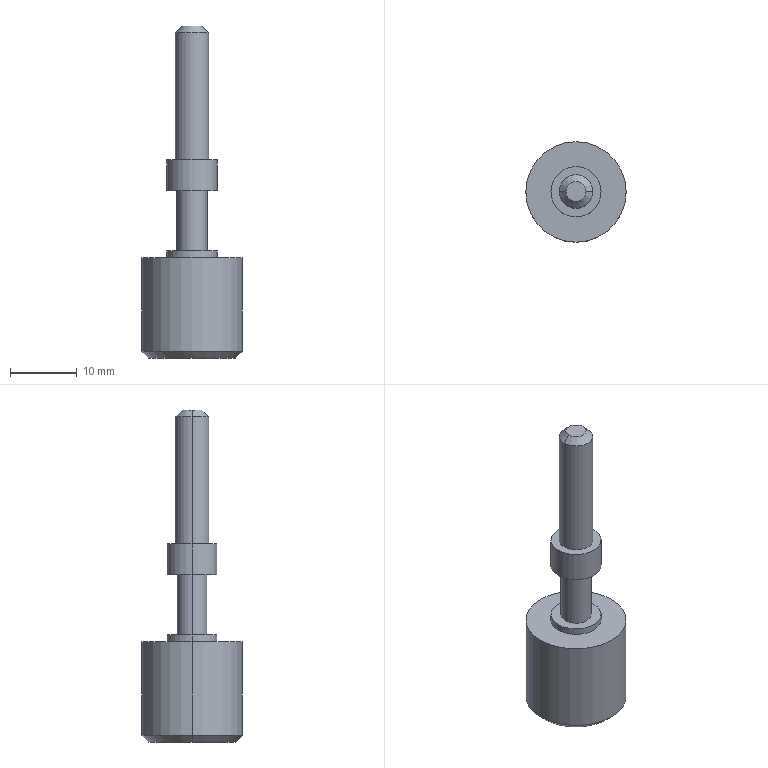Part | STEP file | 001-005-PAZ32_M5_L20 | 1 solid | 27 faces | box 15 x 15 x 49.6 mm | volume 3017 mm3 | plane 13 | cylinder 10 | cone 4 | commonest cylinder face diameters 7.5 x4 4.5 x2 5 x2 15 x2